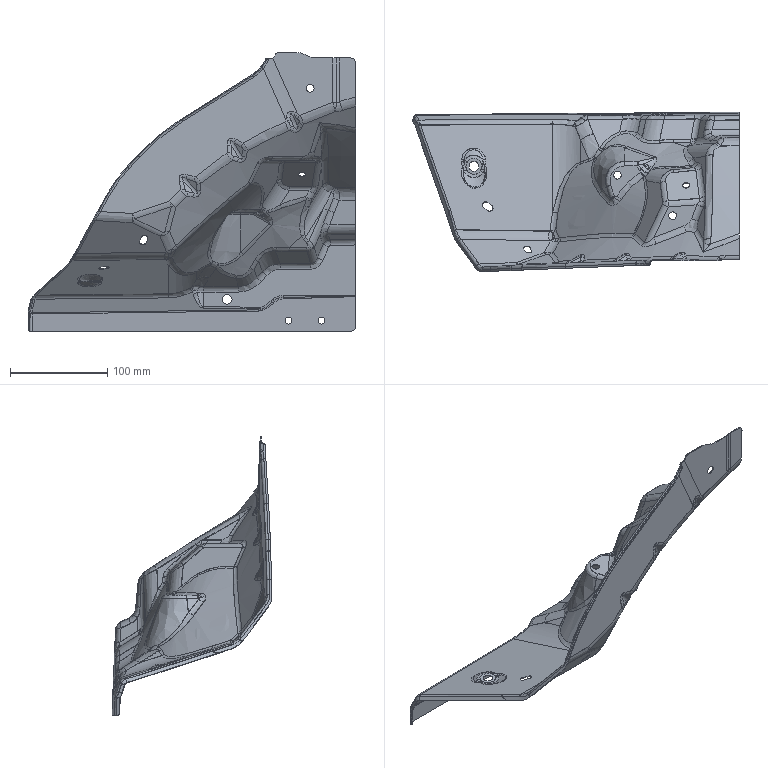Part | 1 solid | 642 faces | box 336.127 x 163.982 x 286.445 mm | volume 80248 mm3 | spline 394 | cylinder 152 | plane 70 | sphere 22 | other 4 | commonest cylinder face diameters 16 x21 10 x16 17.6 x12 8.4 x9 14.4 x9 4.4 x8